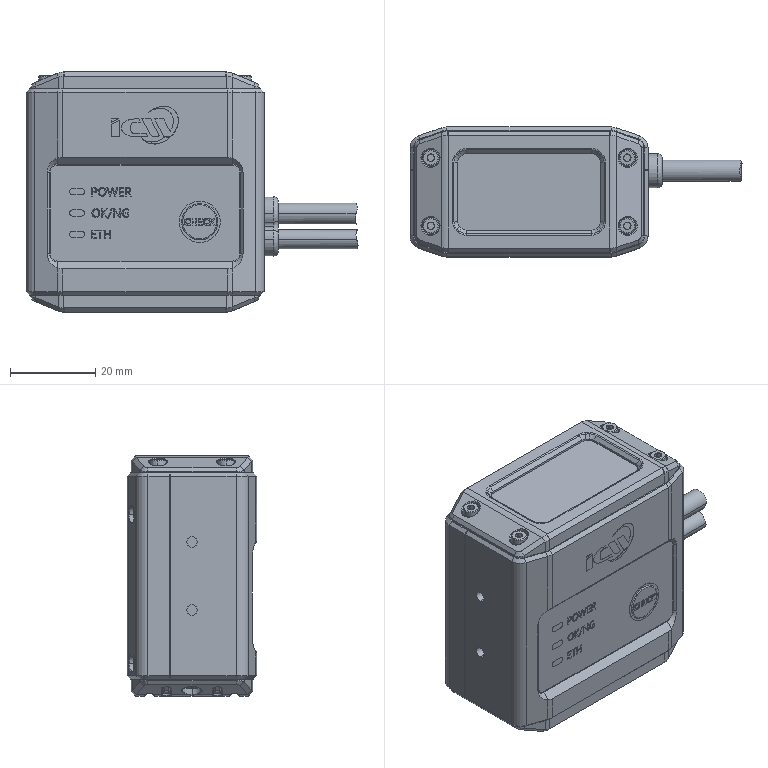Part | SolidWorks | 23 solids | 2770 faces | box 78.091 x 30.5 x 56.5 mm | volume 41886 mm3 | cylinder 970 | plane 871 | spline 492 | cone 210 | torus 169 | sphere 58 | commonest cylinder face diameters 1.713 x174 1.376 x124 4 x107 1 x68 0.4 x52 2 x46